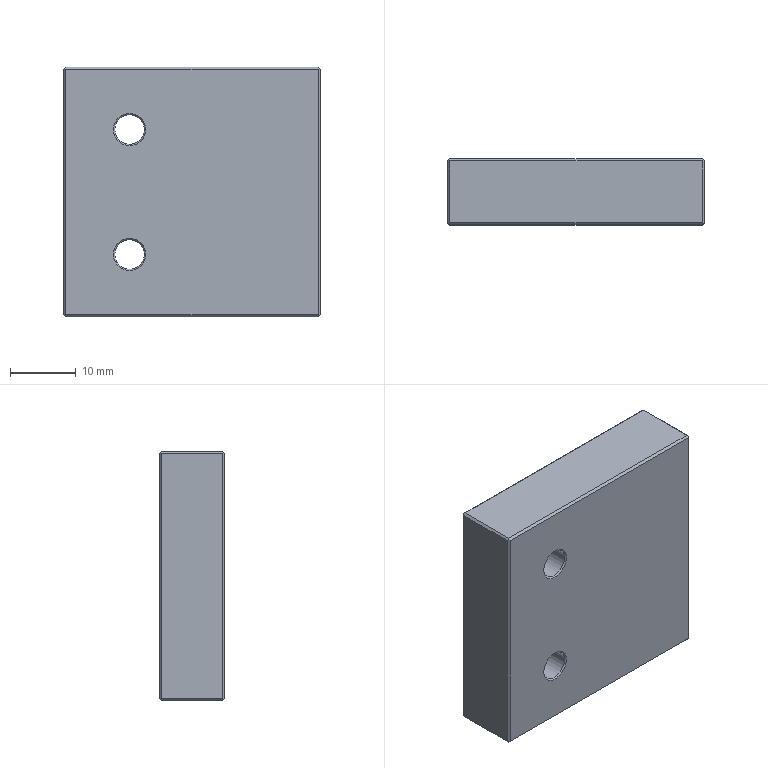Part | NX | 1 solid | 42 faces | box 39 x 10 x 38 mm | volume 14394 mm3 | plane 18 | cylinder 12 | cone 12 | commonest cylinder face diameters 2.5 x8 4.5 x4
STEP:
#1=CARTESIAN_POINT('',(-67.3,-35.,40.2));
#2=VERTEX_POINT('',#1);
#3=CARTESIAN_POINT('',(-67.3,-35.,2.8));
#4=VERTEX_POINT('',#3);
#5=CARTESIAN_POINT('',(-67.3,-35.,21.5));
#6=DIRECTION('',(0.,0.,-1.));
#7=VECTOR('',#6,1000.);
#8=LINE('',#5,#7);
#9=EDGE_CURVE('',#2,#4,#8,.T.);
#10=ORIENTED_EDGE('',*,*,#9,.F.);
#11=CARTESIAN_POINT('',(-105.7,-35.,40.2));
#12=VERTEX_POINT('',#11);
#13=CARTESIAN_POINT('',(-86.5,-35.,40.2));
#14=DIRECTION('',(-1.,0.,0.));
#15=VECTOR('',#14,1000.);
#16=LINE('',#13,#15);
#17=EDGE_CURVE('',#2,#12,#16,.T.);
#18=ORIENTED_EDGE('',*,*,#17,.T.);
#19=CARTESIAN_POINT('',(-105.7,-35.,2.8));
#20=VERTEX_POINT('',#19);
#21=CARTESIAN_POINT('',(-105.7,-35.,21.5));
#22=DIRECTION('',(0.,0.,-1.));
#23=VECTOR('',#22,1000.);
#24=LINE('',#21,#23);
#25=EDGE_CURVE('',#12,#20,#24,.T.);
#26=ORIENTED_EDGE('',*,*,#25,.T.);
#27=CARTESIAN_POINT('',(-86.5,-35.,2.8));
#28=DIRECTION('',(1.,0.,0.));
#29=VECTOR('',#28,1000.);
#30=LINE('',#27,#29);
#31=EDGE_CURVE('',#20,#4,#30,.T.);
#32=ORIENTED_EDGE('',*,*,#31,.T.);
#33=EDGE_LOOP('',(#10,#18,#26,#32));
#34=FACE_BOUND('',#33,.T.);
#35=CARTESIAN_POINT('',(-93.55,-35.,31.));
#36=VERTEX_POINT('',#35);
#37=CARTESIAN_POINT('',(-98.45,-35.,31.));
#38=VERTEX_POINT('',#37);
#39=CARTESIAN_POINT('',(-96.,-35.,31.));
#40=DIRECTION('',(0.,-1.,0.));
#41=DIRECTION('',(-1.,0.,0.));
#42=AXIS2_PLACEMENT_3D('',#39,#40,#41);
#43=CIRCLE('',#42,2.45);
#44=EDGE_CURVE('',#36,#38,#43,.T.);
#45=ORIENTED_EDGE('',*,*,#44,.F.);
#46=CARTESIAN_POINT('',(-96.,-35.,31.));
#47=DIRECTION('',(0.,-1.,0.));
#48=DIRECTION('',(-1.,0.,0.));
#49=AXIS2_PLACEMENT_3D('',#46,#47,#48);
#50=CIRCLE('',#49,2.45);
#51=EDGE_CURVE('',#38,#36,#50,.T.);
#52=ORIENTED_EDGE('',*,*,#51,.F.);
#53=EDGE_LOOP('',(#45,#52));
#54=FACE_BOUND('',#53,.T.);
#55=CARTESIAN_POINT('',(-93.55,-35.,12.));
#56=VERTEX_POINT('',#55);
#57=CARTESIAN_POINT('',(-98.45,-35.,12.));
#58=VERTEX_POINT('',#57);
#59=CARTESIAN_POINT('',(-96.,-35.,12.));
#60=DIRECTION('',(0.,-1.,0.));
#61=DIRECTION('',(-1.,0.,0.));
#62=AXIS2_PLACEMENT_3D('',#59,#60,#61);
#63=CIRCLE('',#62,2.45);
#64=EDGE_CURVE('',#56,#58,#63,.T.);
#65=ORIENTED_EDGE('',*,*,#64,.F.);
#66=CARTESIAN_POINT('',(-96.,-35.,12.));
#67=DIRECTION('',(0.,-1.,0.));
#68=DIRECTION('',(-1.,0.,0.));
#69=AXIS2_PLACEMENT_3D('',#66,#67,#68);
#70=CIRCLE('',#69,2.45);
#71=EDGE_CURVE('',#58,#56,#70,.T.);
#72=ORIENTED_EDGE('',*,*,#71,.F.);
#73=EDGE_LOOP('',(#65,#72));
#74=FACE_BOUND('',#73,.T.);
#75=CARTESIAN_POINT('',(0.,-35.,0.));
#76=DIRECTION('',(0.,1.,0.));
#77=DIRECTION('',(1.,0.,0.));
#78=AXIS2_PLACEMENT_3D('',#75,#76,#77);
#79=PLANE('',#78);
#80=ADVANCED_FACE('',(#34,#54,#74),#79,.F.);
#81=CARTESIAN_POINT('',(-105.7,-25.,2.8));
#82=VERTEX_POINT('',#81);
#83=CARTESIAN_POINT('',(-105.7,-25.,40.2));
#84=VERTEX_POINT('',#83);
#85=CARTESIAN_POINT('',(-105.7,-25.,21.5));
#86=DIRECTION('',(0.,0.,1.));
#87=VECTOR('',#86,1000.);
#88=LINE('',#85,#87);
#89=EDGE_CURVE('',#82,#84,#88,.T.);
#90=ORIENTED_EDGE('',*,*,#89,.T.);
#91=CARTESIAN_POINT('',(-67.3,-25.,40.2));
#92=VERTEX_POINT('',#91);
#93=CARTESIAN_POINT('',(-86.5,-25.,40.2));
#94=DIRECTION('',(-1.,0.,0.));
#95=VECTOR('',#94,1000.);
#96=LINE('',#93,#95);
#97=EDGE_CURVE('',#92,#84,#96,.T.);
#98=ORIENTED_EDGE('',*,*,#97,.F.);
#99=CARTESIAN_POINT('',(-67.3,-25.,2.8));
#100=VERTEX_POINT('',#99);
#101=CARTESIAN_POINT('',(-67.3,-25.,21.5));
#102=DIRECTION('',(0.,0.,1.));
#103=VECTOR('',#102,1000.);
#104=LINE('',#101,#103);
#105=EDGE_CURVE('',#100,#92,#104,.T.);
#106=ORIENTED_EDGE('',*,*,#105,.F.);
#107=CARTESIAN_POINT('',(-86.5,-25.,2.8));
#108=DIRECTION('',(1.,0.,0.));
#109=VECTOR('',#108,1000.);
#110=LINE('',#107,#109);
#111=EDGE_CURVE('',#82,#100,#110,.T.);
#112=ORIENTED_EDGE('',*,*,#111,.F.);
#113=EDGE_LOOP('',(#90,#98,#106,#112));
#114=FACE_BOUND('',#113,.T.);
#115=CARTESIAN_POINT('',(-93.75,-25.,12.));
#116=VERTEX_POINT('',#115);
#117=CARTESIAN_POINT('',(-98.25,-25.,12.));
#118=VERTEX_POINT('',#117);
#119=CARTESIAN_POINT('',(-96.,-25.,12.));
#120=DIRECTION('',(0.,-1.,0.));
#121=DIRECTION('',(-1.,0.,0.));
#122=AXIS2_PLACEMENT_3D('',#119,#120,#121);
#123=CIRCLE('',#122,2.25);
#124=EDGE_CURVE('',#116,#118,#123,.T.);
#125=ORIENTED_EDGE('',*,*,#124,.T.);
#126=CARTESIAN_POINT('',(-96.,-25.,12.));
#127=DIRECTION('',(0.,-1.,0.));
#128=DIRECTION('',(-1.,0.,0.));
#129=AXIS2_PLACEMENT_3D('',#126,#127,#128);
#130=CIRCLE('',#129,2.25);
#131=EDGE_CURVE('',#118,#116,#130,.T.);
#132=ORIENTED_EDGE('',*,*,#131,.T.);
#133=EDGE_LOOP('',(#125,#132));
#134=FACE_BOUND('',#133,.T.);
#135=CARTESIAN_POINT('',(-93.75,-25.,31.));
#136=VERTEX_POINT('',#135);
#137=CARTESIAN_POINT('',(-98.25,-25.,31.));
#138=VERTEX_POINT('',#137);
#139=CARTESIAN_POINT('',(-96.,-25.,31.));
#140=DIRECTION('',(0.,-1.,0.));
#141=DIRECTION('',(-1.,0.,0.));
#142=AXIS2_PLACEMENT_3D('',#139,#140,#141);
#143=CIRCLE('',#142,2.25);
#144=EDGE_CURVE('',#136,#138,#143,.T.);
#145=ORIENTED_EDGE('',*,*,#144,.T.);
#146=CARTESIAN_POINT('',(-96.,-25.,31.));
#147=DIRECTION('',(0.,-1.,0.));
#148=DIRECTION('',(-1.,0.,0.));
#149=AXIS2_PLACEMENT_3D('',#146,#147,#148);
#150=CIRCLE('',#149,2.25);
#151=EDGE_CURVE('',#138,#136,#150,.T.);
#152=ORIENTED_EDGE('',*,*,#151,.T.);
#153=EDGE_LOOP('',(#145,#152));
#154=FACE_BOUND('',#153,.T.);
#155=CARTESIAN_POINT('',(-8.5,-25.,1.2));
#156=DIRECTION('',(0.,-1.,0.));
#157=DIRECTION('',(-1.,0.,0.));
#158=AXIS2_PLACEMENT_3D('',#155,#156,#157);
#159=PLANE('',#158);
#160=ADVANCED_FACE('',(#114,#134,#154),#159,.F.);
#161=CARTESIAN_POINT('',(-106.,-25.3,2.8));
#162=VERTEX_POINT('',#161);
#163=CARTESIAN_POINT('',(-106.,-25.3,40.2));
#164=VERTEX_POINT('',#163);
#165=CARTESIAN_POINT('',(-106.,-25.3,21.5));
#166=DIRECTION('',(0.,0.,1.));
#167=VECTOR('',#166,1000.);
#168=LINE('',#165,#167);
#169=EDGE_CURVE('',#162,#164,#168,.T.);
#170=ORIENTED_EDGE('',*,*,#169,.F.);
#171=CARTESIAN_POINT('',(-106.,-34.7,2.8));
#172=VERTEX_POINT('',#171);
#173=CARTESIAN_POINT('',(-106.,-30.,2.8));
#174=DIRECTION('',(0.,1.,0.));
#175=VECTOR('',#174,1000.);
#176=LINE('',#173,#175);
#177=EDGE_CURVE('',#172,#162,#176,.T.);
#178=ORIENTED_EDGE('',*,*,#177,.F.);
#179=CARTESIAN_POINT('',(-106.,-34.7,40.2));
#180=VERTEX_POINT('',#179);
#181=CARTESIAN_POINT('',(-106.,-34.7,21.5));
#182=DIRECTION('',(0.,0.,-1.));
#183=VECTOR('',#182,1000.);
#184=LINE('',#181,#183);
#185=EDGE_CURVE('',#180,#172,#184,.T.);
#186=ORIENTED_EDGE('',*,*,#185,.F.);
#187=CARTESIAN_POINT('',(-106.,-30.,40.2));
#188=DIRECTION('',(0.,-1.,0.));
#189=VECTOR('',#188,1000.);
#190=LINE('',#187,#189);
#191=EDGE_CURVE('',#164,#180,#190,.T.);
#192=ORIENTED_EDGE('',*,*,#191,.F.);
#193=EDGE_LOOP('',(#170,#178,#186,#192));
#194=FACE_BOUND('',#193,.T.);
#195=CARTESIAN_POINT('',(-106.,0.,0.));
#196=DIRECTION('',(1.,0.,0.));
#197=DIRECTION('',(0.,1.,0.));
#198=AXIS2_PLACEMENT_3D('',#195,#196,#197);
#199=PLANE('',#198);
#200=ADVANCED_FACE('',(#194),#199,.F.);
#201=CARTESIAN_POINT('',(-67.3,-25.3,2.5));
#202=VERTEX_POINT('',#201);
#203=CARTESIAN_POINT('',(-67.3,-34.7,2.5));
#204=VERTEX_POINT('',#203);
#205=CARTESIAN_POINT('',(-67.3,0.,2.5));
#206=DIRECTION('',(0.,-1.,0.));
#207=VECTOR('',#206,1000.);
#208=LINE('',#205,#207);
#209=EDGE_CURVE('',#202,#204,#208,.T.);
#210=ORIENTED_EDGE('',*,*,#209,.T.);
#211=CARTESIAN_POINT('',(-105.7,-34.7,2.5));
#212=VERTEX_POINT('',#211);
#213=CARTESIAN_POINT('',(-86.5,-34.7,2.5));
#214=DIRECTION('',(1.,0.,0.));
#215=VECTOR('',#214,1000.);
#216=LINE('',#213,#215);
#217=EDGE_CURVE('',#212,#204,#216,.T.);
#218=ORIENTED_EDGE('',*,*,#217,.F.);
#219=CARTESIAN_POINT('',(-105.7,-25.3,2.5));
#220=VERTEX_POINT('',#219);
#221=CARTESIAN_POINT('',(-105.7,-30.,2.5));
#222=DIRECTION('',(0.,1.,0.));
#223=VECTOR('',#222,1000.);
#224=LINE('',#221,#223);
#225=EDGE_CURVE('',#212,#220,#224,.T.);
#226=ORIENTED_EDGE('',*,*,#225,.T.);
#227=CARTESIAN_POINT('',(-86.5,-25.3,2.5));
#228=DIRECTION('',(1.,0.,0.));
#229=VECTOR('',#228,1000.);
#230=LINE('',#227,#229);
#231=EDGE_CURVE('',#220,#202,#230,.T.);
#232=ORIENTED_EDGE('',*,*,#231,.T.);
#233=EDGE_LOOP('',(#210,#218,#226,#232));
#234=FACE_BOUND('',#233,.T.);
#235=CARTESIAN_POINT('',(-71.3,-31.,2.5));
#236=VERTEX_POINT('',#235);
#237=CARTESIAN_POINT('',(-74.7,-31.,2.5));
#238=VERTEX_POINT('',#237);
#239=CARTESIAN_POINT('',(-73.,-31.,2.5));
#240=DIRECTION('',(0.,0.,-1.));
#241=DIRECTION('',(-1.,0.,0.));
#242=AXIS2_PLACEMENT_3D('',#239,#240,#241);
#243=CIRCLE('',#242,1.7);
#244=EDGE_CURVE('',#236,#238,#243,.T.);
#245=ORIENTED_EDGE('',*,*,#244,.F.);
#246=CARTESIAN_POINT('',(-73.,-31.,2.5));
#247=DIRECTION('',(0.,0.,-1.));
#248=DIRECTION('',(-1.,0.,0.));
#249=AXIS2_PLACEMENT_3D('',#246,#247,#248);
#250=CIRCLE('',#249,1.7);
#251=EDGE_CURVE('',#238,#236,#250,.T.);
#252=ORIENTED_EDGE('',*,*,#251,.F.);
#253=EDGE_LOOP('',(#245,#252));
#254=FACE_BOUND('',#253,.T.);
#255=CARTESIAN_POINT('',(-78.3,-31.,2.5));
#256=VERTEX_POINT('',#255);
#257=CARTESIAN_POINT('',(-81.7,-31.,2.5));
#258=VERTEX_POINT('',#257);
#259=CARTESIAN_POINT('',(-80.,-31.,2.5));
#260=DIRECTION('',(0.,0.,-1.));
#261=DIRECTION('',(-1.,0.,0.));
#262=AXIS2_PLACEMENT_3D('',#259,#260,#261);
#263=CIRCLE('',#262,1.7);
#264=EDGE_CURVE('',#256,#258,#263,.T.);
#265=ORIENTED_EDGE('',*,*,#264,.F.);
#266=CARTESIAN_POINT('',(-80.,-31.,2.5));
#267=DIRECTION('',(0.,0.,-1.));
#268=DIRECTION('',(-1.,0.,0.));
#269=AXIS2_PLACEMENT_3D('',#266,#267,#268);
#270=CIRCLE('',#269,1.7);
#271=EDGE_CURVE('',#258,#256,#270,.T.);
#272=ORIENTED_EDGE('',*,*,#271,.F.);
#273=EDGE_LOOP('',(#265,#272));
#274=FACE_BOUND('',#273,.T.);
#275=CARTESIAN_POINT('',(-35.,0.,2.5));
#276=DIRECTION('',(0.,0.,1.));
#277=DIRECTION('',(1.,0.,0.));
#278=AXIS2_PLACEMENT_3D('',#275,#276,#277);
#279=PLANE('',#278);
#280=ADVANCED_FACE('',(#234,#254,#274),#279,.F.);
#281=CARTESIAN_POINT('',(-105.7,-25.3,40.5));
#282=VERTEX_POINT('',#281);
#283=CARTESIAN_POINT('',(-105.7,-34.7,40.5));
#284=VERTEX_POINT('',#283);
#285=CARTESIAN_POINT('',(-105.7,-30.,40.5));
#286=DIRECTION('',(0.,-1.,0.));
#287=VECTOR('',#286,1000.);
#288=LINE('',#285,#287);
#289=EDGE_CURVE('',#282,#284,#288,.T.);
#290=ORIENTED_EDGE('',*,*,#289,.F.);
#291=CARTESIAN_POINT('',(-105.85,-25.15,40.35));
#292=VERTEX_POINT('',#291);
#293=CARTESIAN_POINT('',(-131.,0.,15.2));
#294=DIRECTION('',(0.5774,-0.5774,0.5774));
#295=VECTOR('',#294,1000.);
#296=LINE('',#293,#295);
#297=EDGE_CURVE('',#292,#282,#296,.T.);
#298=ORIENTED_EDGE('',*,*,#297,.F.);
#299=CARTESIAN_POINT('',(-146.2,-65.5,0.));
#300=DIRECTION('',(0.5774,0.5774,0.5774));
#301=VECTOR('',#300,1000.);
#302=LINE('',#299,#301);
#303=EDGE_CURVE('',#164,#292,#302,.T.);
#304=ORIENTED_EDGE('',*,*,#303,.F.);
#305=ORIENTED_EDGE('',*,*,#191,.T.);
#306=CARTESIAN_POINT('',(-105.85,-34.85,40.35));
#307=VERTEX_POINT('',#306);
#308=CARTESIAN_POINT('',(-146.2,5.5,0.));
#309=DIRECTION('',(-0.5774,0.5774,-0.5774));
#310=VECTOR('',#309,1000.);
#311=LINE('',#308,#310);
#312=EDGE_CURVE('',#307,#180,#311,.T.);
#313=ORIENTED_EDGE('',*,*,#312,.F.);
#314=CARTESIAN_POINT('',(-146.2,-75.2,0.));
#315=DIRECTION('',(-0.5774,-0.5774,-0.5774));
#316=VECTOR('',#315,1000.);
#317=LINE('',#314,#316);
#318=EDGE_CURVE('',#284,#307,#317,.T.);
#319=ORIENTED_EDGE('',*,*,#318,.F.);
#320=EDGE_LOOP('',(#290,#298,#304,#305,#313,#319));
#321=FACE_BOUND('',#320,.T.);
#322=CARTESIAN_POINT('',(-105.85,-30.,40.35));
#323=DIRECTION('',(-0.7071,0.,0.7071));
#324=DIRECTION('',(0.,1.,0.));
#325=AXIS2_PLACEMENT_3D('',#322,#323,#324);
#326=PLANE('',#325);
#327=ADVANCED_FACE('',(#321),#326,.T.);
#328=ORIENTED_EDGE('',*,*,#289,.T.);
#329=CARTESIAN_POINT('',(-67.3,-34.7,40.5));
#330=VERTEX_POINT('',#329);
#331=CARTESIAN_POINT('',(-86.5,-34.7,40.5));
#332=DIRECTION('',(-1.,0.,0.));
#333=VECTOR('',#332,1000.);
#334=LINE('',#331,#333);
#335=EDGE_CURVE('',#330,#284,#334,.T.);
#336=ORIENTED_EDGE('',*,*,#335,.F.);
#337=CARTESIAN_POINT('',(-67.3,-25.3,40.5));
#338=VERTEX_POINT('',#337);
#339=CARTESIAN_POINT('',(-67.3,-30.,40.5));
#340=DIRECTION('',(0.,1.,0.));
#341=VECTOR('',#340,1000.);
#342=LINE('',#339,#341);
#343=EDGE_CURVE('',#330,#338,#342,.T.);
#344=ORIENTED_EDGE('',*,*,#343,.T.);
#345=CARTESIAN_POINT('',(-86.5,-25.3,40.5));
#346=DIRECTION('',(-1.,0.,0.));
#347=VECTOR('',#346,1000.);
#348=LINE('',#345,#347);
#349=EDGE_CURVE('',#338,#282,#348,.T.);
#350=ORIENTED_EDGE('',*,*,#349,.T.);
#351=EDGE_LOOP('',(#328,#336,#344,#350));
#352=FACE_BOUND('',#351,.T.);
#353=CARTESIAN_POINT('',(-20.5,7.5,40.5));
#354=DIRECTION('',(0.,0.,-1.));
#355=DIRECTION('',(0.,-1.,0.));
#356=AXIS2_PLACEMENT_3D('',#353,#354,#355);
#357=PLANE('',#356);
#358=ADVANCED_FACE('',(#352),#357,.F.);
#359=CARTESIAN_POINT('',(-78.75,-31.,2.76));
#360=VERTEX_POINT('',#359);
#361=CARTESIAN_POINT('',(-81.25,-31.,2.76));
#362=VERTEX_POINT('',#361);
#363=CARTESIAN_POINT('',(-80.,-31.,2.76));
#364=DIRECTION('',(0.,0.,-1.));
#365=DIRECTION('',(-1.,0.,0.));
#366=AXIS2_PLACEMENT_3D('',#363,#364,#365);
#367=CIRCLE('',#366,1.25);
#368=EDGE_CURVE('',#360,#362,#367,.T.);
#369=ORIENTED_EDGE('',*,*,#368,.T.);
#370=CARTESIAN_POINT('',(-81.25,-31.,8.5));
#371=VERTEX_POINT('',#370);
#372=CARTESIAN_POINT('',(-81.25,-31.,2.5));
#373=DIRECTION('',(0.,0.,-1.));
#374=VECTOR('',#373,1000.);
#375=LINE('',#372,#374);
#376=EDGE_CURVE('',#362,#371,#375,.F.);
#377=ORIENTED_EDGE('',*,*,#376,.T.);
#378=CARTESIAN_POINT('',(-78.75,-31.,8.5));
#379=VERTEX_POINT('',#378);
#380=CARTESIAN_POINT('',(-80.,-31.,8.5));
#381=DIRECTION('',(0.,0.,-1.));
#382=DIRECTION('',(-1.,0.,0.));
#383=AXIS2_PLACEMENT_3D('',#380,#381,#382);
#384=CIRCLE('',#383,1.25);
#385=EDGE_CURVE('',#379,#371,#384,.T.);
#386=ORIENTED_EDGE('',*,*,#385,.F.);
#387=CARTESIAN_POINT('',(-78.75,-31.,2.5));
#388=DIRECTION('',(0.,0.,-1.));
#389=VECTOR('',#388,1000.);
#390=LINE('',#387,#389);
#391=EDGE_CURVE('',#360,#379,#390,.F.);
#392=ORIENTED_EDGE('',*,*,#391,.F.);
#393=EDGE_LOOP('',(#369,#377,#386,#392));
#394=FACE_BOUND('',#393,.T.);
#395=CARTESIAN_POINT('',(-80.,-31.,2.5));
#396=DIRECTION('',(0.,0.,-1.));
#397=DIRECTION('',(-1.,0.,0.));
#398=AXIS2_PLACEMENT_3D('',#395,#396,#397);
#399=CYLINDRICAL_SURFACE('',#398,1.25);
#400=ADVANCED_FACE('',(#394),#399,.F.);
#401=ORIENTED_EDGE('',*,*,#385,.T.);
#402=CARTESIAN_POINT('',(-81.25,-31.,11.5));
#403=VERTEX_POINT('',#402);
#404=CARTESIAN_POINT('',(-81.25,-31.,2.5));
#405=DIRECTION('',(0.,0.,-1.));
#406=VECTOR('',#405,1000.);
#407=LINE('',#404,#406);
#408=EDGE_CURVE('',#371,#403,#407,.F.);
#409=ORIENTED_EDGE('',*,*,#408,.T.);
#410=CARTESIAN_POINT('',(-78.75,-31.,11.5));
#411=VERTEX_POINT('',#410);
#412=CARTESIAN_POINT('',(-80.,-31.,11.5));
#413=DIRECTION('',(0.,0.,-1.));
#414=DIRECTION('',(-1.,0.,0.));
#415=AXIS2_PLACEMENT_3D('',#412,#413,#414);
#416=CIRCLE('',#415,1.25);
#417=EDGE_CURVE('',#411,#403,#416,.T.);
#418=ORIENTED_EDGE('',*,*,#417,.F.);
#419=CARTESIAN_POINT('',(-78.75,-31.,2.5));
#420=DIRECTION('',(0.,0.,-1.));
#421=VECTOR('',#420,1000.);
#422=LINE('',#419,#421);
#423=EDGE_CURVE('',#379,#411,#422,.F.);
#424=ORIENTED_EDGE('',*,*,#423,.F.);
#425=EDGE_LOOP('',(#401,#409,#418,#424));
#426=FACE_BOUND('',#425,.T.);
#427=CARTESIAN_POINT('',(-80.,-31.,2.5));
#428=DIRECTION('',(0.,0.,-1.));
#429=DIRECTION('',(-1.,0.,0.));
#430=AXIS2_PLACEMENT_3D('',#427,#428,#429);
#431=CYLINDRICAL_SURFACE('',#430,1.25);
#432=ADVANCED_FACE('',(#426),#431,.F.);
#433=ORIENTED_EDGE('',*,*,#417,.T.);
#434=CARTESIAN_POINT('',(-80.,-31.,12.251));
#435=VERTEX_POINT('',#434);
#436=CARTESIAN_POINT('',(-81.25,-31.,11.5));
#437=DIRECTION('',(-0.8572,0.,-0.515));
#438=VECTOR('',#437,1000.);
#439=LINE('',#436,#438);
#440=EDGE_CURVE('',#435,#403,#439,.T.);
#441=ORIENTED_EDGE('',*,*,#440,.F.);
#442=CARTESIAN_POINT('',(-78.75,-31.,11.5));
#443=DIRECTION('',(0.8572,0.,-0.515));
#444=VECTOR('',#443,1000.);
#445=LINE('',#442,#444);
#446=EDGE_CURVE('',#435,#411,#445,.T.);
#447=ORIENTED_EDGE('',*,*,#446,.T.);
#448=EDGE_LOOP('',(#433,#441,#447));
#449=FACE_BOUND('',#448,.T.);
#450=CARTESIAN_POINT('',(-80.,-31.,11.5));
#451=DIRECTION('',(0.,0.,-1.));
#452=DIRECTION('',(-1.,0.,0.));
#453=AXIS2_PLACEMENT_3D('',#450,#451,#452);
#454=CONICAL_SURFACE('',#453,1.25,1.03);
#455=ADVANCED_FACE('',(#449),#454,.F.);
#456=CARTESIAN_POINT('',(-93.75,-34.8,31.));
#457=VERTEX_POINT('',#456);
#458=CARTESIAN_POINT('',(-98.25,-34.8,31.));
#459=VERTEX_POINT('',#458);
#460=CARTESIAN_POINT('',(-96.,-34.8,31.));
#461=DIRECTION('',(0.,-1.,0.));
#462=DIRECTION('',(-1.,0.,0.));
#463=AXIS2_PLACEMENT_3D('',#460,#461,#462);
#464=CIRCLE('',#463,2.25);
#465=EDGE_CURVE('',#457,#459,#464,.T.);
#466=ORIENTED_EDGE('',*,*,#465,.T.);
#467=CARTESIAN_POINT('',(-98.25,-35.,31.));
#468=DIRECTION('',(0.,-1.,0.));
#469=VECTOR('',#468,1000.);
#470=LINE('',#467,#469);
#471=EDGE_CURVE('',#459,#138,#470,.F.);
#472=ORIENTED_EDGE('',*,*,#471,.T.);
#473=ORIENTED_EDGE('',*,*,#144,.F.);
#474=CARTESIAN_POINT('',(-93.75,-35.,31.));
#475=DIRECTION('',(0.,-1.,0.));
#476=VECTOR('',#475,1000.);
#477=LINE('',#474,#476);
#478=EDGE_CURVE('',#457,#136,#477,.F.);
#479=ORIENTED_EDGE('',*,*,#478,.F.);
#480=EDGE_LOOP('',(#466,#472,#473,#479));
#481=FACE_BOUND('',#480,.T.);
#482=CARTESIAN_POINT('',(-96.,-35.,31.));
#483=DIRECTION('',(0.,-1.,0.));
#484=DIRECTION('',(-1.,0.,0.));
#485=AXIS2_PLACEMENT_3D('',#482,#483,#484);
#486=CYLINDRICAL_SURFACE('',#485,2.25);
#487=ADVANCED_FACE('',(#481),#486,.F.);
#488=CARTESIAN_POINT('',(-71.75,-31.,2.76));
#489=VERTEX_POINT('',#488);
#490=CARTESIAN_POINT('',(-74.25,-31.,2.76));
#491=VERTEX_POINT('',#490);
#492=CARTESIAN_POINT('',(-73.,-31.,2.76));
#493=DIRECTION('',(0.,0.,-1.));
#494=DIRECTION('',(-1.,0.,0.));
#495=AXIS2_PLACEMENT_3D('',#492,#493,#494);
#496=CIRCLE('',#495,1.25);
#497=EDGE_CURVE('',#489,#491,#496,.T.);
#498=ORIENTED_EDGE('',*,*,#497,.T.);
#499=CARTESIAN_POINT('',(-74.25,-31.,8.5));
#500=VERTEX_POINT('',#499);
#501=CARTESIAN_POINT('',(-74.25,-31.,2.5));
#502=DIRECTION('',(0.,0.,-1.));
#503=VECTOR('',#502,1000.);
#504=LINE('',#501,#503);
#505=EDGE_CURVE('',#491,#500,#504,.F.);
#506=ORIENTED_EDGE('',*,*,#505,.T.);
#507=CARTESIAN_POINT('',(-71.75,-31.,8.5));
#508=VERTEX_POINT('',#507);
#509=CARTESIAN_POINT('',(-73.,-31.,8.5));
#510=DIRECTION('',(0.,0.,-1.));
#511=DIRECTION('',(-1.,0.,0.));
#512=AXIS2_PLACEMENT_3D('',#509,#510,#511);
#513=CIRCLE('',#512,1.25);
#514=EDGE_CURVE('',#508,#500,#513,.T.);
#515=ORIENTED_EDGE('',*,*,#514,.F.);
#516=CARTESIAN_POINT('',(-71.75,-31.,2.5));
#517=DIRECTION('',(0.,0.,-1.));
#518=VECTOR('',#517,1000.);
#519=LINE('',#516,#518);
#520=EDGE_CURVE('',#489,#508,#519,.F.);
#521=ORIENTED_EDGE('',*,*,#520,.F.);
#522=EDGE_LOOP('',(#498,#506,#515,#521));
#523=FACE_BOUND('',#522,.T.);
#524=CARTESIAN_POINT('',(-73.,-31.,2.5));
#525=DIRECTION('',(0.,0.,-1.));
#526=DIRECTION('',(-1.,0.,0.));
#527=AXIS2_PLACEMENT_3D('',#524,#525,#526);
#528=CYLINDRICAL_SURFACE('',#527,1.25);
#529=ADVANCED_FACE('',(#523),#528,.F.);
#530=ORIENTED_EDGE('',*,*,#514,.T.);
#531=CARTESIAN_POINT('',(-74.25,-31.,11.5));
#532=VERTEX_POINT('',#531);
#533=CARTESIAN_POINT('',(-74.25,-31.,2.5));
#534=DIRECTION('',(0.,0.,-1.));
#535=VECTOR('',#534,1000.);
#536=LINE('',#533,#535);
#537=EDGE_CURVE('',#500,#532,#536,.F.);
#538=ORIENTED_EDGE('',*,*,#537,.T.);
#539=CARTESIAN_POINT('',(-71.75,-31.,11.5));
#540=VERTEX_POINT('',#539);
#541=CARTESIAN_POINT('',(-73.,-31.,11.5));
#542=DIRECTION('',(0.,0.,-1.));
#543=DIRECTION('',(-1.,0.,0.));
#544=AXIS2_PLACEMENT_3D('',#541,#542,#543);
#545=CIRCLE('',#544,1.25);
#546=EDGE_CURVE('',#540,#532,#545,.T.);
#547=ORIENTED_EDGE('',*,*,#546,.F.);
#548=CARTESIAN_POINT('',(-71.75,-31.,2.5));
#549=DIRECTION('',(0.,0.,-1.));
#550=VECTOR('',#549,1000.);
#551=LINE('',#548,#550);
#552=EDGE_CURVE('',#508,#540,#551,.F.);
#553=ORIENTED_EDGE('',*,*,#552,.F.);
#554=EDGE_LOOP('',(#530,#538,#547,#553));
#555=FACE_BOUND('',#554,.T.);
#556=CARTESIAN_POINT('',(-73.,-31.,2.5));
#557=DIRECTION('',(0.,0.,-1.));
#558=DIRECTION('',(-1.,0.,0.));
#559=AXIS2_PLACEMENT_3D('',#556,#557,#558);
#560=CYLINDRICAL_SURFACE('',#559,1.25);
#561=ADVANCED_FACE('',(#555),#560,.F.);
#562=ORIENTED_EDGE('',*,*,#546,.T.);
#563=CARTESIAN_POINT('',(-73.,-31.,12.251));
#564=VERTEX_POINT('',#563);
#565=CARTESIAN_POINT('',(-74.25,-31.,11.5));
#566=DIRECTION('',(-0.8572,0.,-0.515));
#567=VECTOR('',#566,1000.);
#568=LINE('',#565,#567);
#569=EDGE_CURVE('',#564,#532,#568,.T.);
#570=ORIENTED_EDGE('',*,*,#569,.F.);
#571=CARTESIAN_POINT('',(-71.75,-31.,11.5));
#572=DIRECTION('',(0.8572,0.,-0.515));
#573=VECTOR('',#572,1000.);
#574=LINE('',#571,#573);
#575=EDGE_CURVE('',#564,#540,#574,.T.);
#576=ORIENTED_EDGE('',*,*,#575,.T.);
#577=EDGE_LOOP('',(#562,#570,#576));
#578=FACE_BOUND('',#577,.T.);
#579=CARTESIAN_POINT('',(-73.,-31.,11.5));
#580=DIRECTION('',(0.,0.,-1.));
#581=DIRECTION('',(-1.,0.,0.));
#582=AXIS2_PLACEMENT_3D('',#579,#580,#581);
#583=CONICAL_SURFACE('',#582,1.25,1.03);
#584=ADVANCED_FACE('',(#578),#583,.F.);
#585=CARTESIAN_POINT('',(-67.,-25.3,2.8));
#586=VERTEX_POINT('',#585);
#587=CARTESIAN_POINT('',(-67.,-34.7,2.8));
#588=VERTEX_POINT('',#587);
#589=CARTESIAN_POINT('',(-67.,0.,2.8));
#590=DIRECTION('',(0.,-1.,0.));
#591=VECTOR('',#590,1000.);
#592=LINE('',#589,#591);
#593=EDGE_CURVE('',#586,#588,#592,.T.);
#594=ORIENTED_EDGE('',*,*,#593,.F.);
#595=CARTESIAN_POINT('',(-67.,-25.3,40.2));
#596=VERTEX_POINT('',#595);
#597=CARTESIAN_POINT('',(-67.,-25.3,0.));
#598=DIRECTION('',(0.,0.,-1.));
#599=VECTOR('',#598,1000.);
#600=LINE('',#597,#599);
#601=EDGE_CURVE('',#596,#586,#600,.T.);
#602=ORIENTED_EDGE('',*,*,#601,.F.);
#603=CARTESIAN_POINT('',(-67.,-34.7,40.2));
#604=VERTEX_POINT('',#603);
#605=CARTESIAN_POINT('',(-67.,-30.,40.2));
#606=DIRECTION('',(0.,1.,0.));
#607=VECTOR('',#606,1000.);
#608=LINE('',#605,#607);
#609=EDGE_CURVE('',#604,#596,#608,.T.);
#610=ORIENTED_EDGE('',*,*,#609,.F.);
#611=CARTESIAN_POINT('',(-67.,-34.7,21.5));
#612=DIRECTION('',(0.,0.,-1.));
#613=VECTOR('',#612,1000.);
#614=LINE('',#611,#613);
#615=EDGE_CURVE('',#604,#588,#614,.T.);
#616=ORIENTED_EDGE('',*,*,#615,.T.);
#617=EDGE_LOOP('',(#594,#602,#610,#616));
#618=FACE_BOUND('',#617,.T.);
#619=CARTESIAN_POINT('',(-67.,-38.5,5.));
#620=DIRECTION('',(1.,0.,0.));
#621=DIRECTION('',(0.,1.,0.));
#622=AXIS2_PLACEMENT_3D('',#619,#620,#621);
#623=PLANE('',#622);
#624=ADVANCED_FACE('',(#618),#623,.T.);
#625=ORIENTED_EDGE('',*,*,#9,.T.);
#626=CARTESIAN_POINT('',(-67.15,-34.85,2.65));
#627=VERTEX_POINT('',#626);
#628=CARTESIAN_POINT('',(0.,32.3,-64.5));
#629=DIRECTION('',(0.5774,0.5774,-0.5774));
#630=VECTOR('',#629,1000.);
#631=LINE('',#628,#630);
#632=EDGE_CURVE('',#4,#627,#631,.T.);
#633=ORIENTED_EDGE('',*,*,#632,.T.);
#634=CARTESIAN_POINT('',(-69.8,-37.5,0.));
#635=DIRECTION('',(-0.5774,-0.5774,-0.5774));
#636=VECTOR('',#635,1000.);
#637=LINE('',#634,#636);
#638=EDGE_CURVE('',#588,#627,#637,.T.);
#639=ORIENTED_EDGE('',*,*,#638,.F.);
#640=ORIENTED_EDGE('',*,*,#615,.F.);
#641=CARTESIAN_POINT('',(-67.15,-34.85,40.35));
#642=VERTEX_POINT('',#641);
#643=CARTESIAN_POINT('',(-26.8,5.5,0.));
#644=DIRECTION('',(0.5774,0.5774,-0.5774));
#645=VECTOR('',#644,1000.);
#646=LINE('',#643,#645);
#647=EDGE_CURVE('',#642,#604,#646,.T.);
#648=ORIENTED_EDGE('',*,*,#647,.F.);
#649=CARTESIAN_POINT('',(0.,32.3,107.5));
#650=DIRECTION('',(-0.5774,-0.5774,-0.5774));
#651=VECTOR('',#650,1000.);
#652=LINE('',#649,#651);
#653=EDGE_CURVE('',#642,#2,#652,.T.);
#654=ORIENTED_EDGE('',*,*,#653,.T.);
#655=EDGE_LOOP('',(#625,#633,#639,#640,#648,#654));
#656=FACE_BOUND('',#655,.T.);
#657=CARTESIAN_POINT('',(-67.15,-34.85,21.5));
#658=DIRECTION('',(-0.7071,0.7071,0.));
#659=DIRECTION('',(0.,0.,1.));
#660=AXIS2_PLACEMENT_3D('',#657,#658,#659);
#661=PLANE('',#660);
#662=ADVANCED_FACE('',(#656),#661,.F.);
#663=ORIENTED_EDGE('',*,*,#593,.T.);
#664=ORIENTED_EDGE('',*,*,#638,.T.);
#665=CARTESIAN_POINT('',(-69.8,-32.2,0.));
#666=DIRECTION('',(0.5774,-0.5774,0.5774));
#667=VECTOR('',#666,1000.);
#668=LINE('',#665,#667);
#669=EDGE_CURVE('',#204,#627,#668,.T.);
#670=ORIENTED_EDGE('',*,*,#669,.F.);
#671=ORIENTED_EDGE('',*,*,#209,.F.);
#672=CARTESIAN_POINT('',(-67.15,-25.15,2.65));
#673=VERTEX_POINT('',#672);
#674=CARTESIAN_POINT('',(-69.8,-27.8,0.));
#675=DIRECTION('',(-0.5774,-0.5774,-0.5774));
#676=VECTOR('',#675,1000.);
#677=LINE('',#674,#676);
#678=EDGE_CURVE('',#673,#202,#677,.T.);
#679=ORIENTED_EDGE('',*,*,#678,.F.);
#680=CARTESIAN_POINT('',(-92.3,0.,-22.5));
#681=DIRECTION('',(0.5774,-0.5774,0.5774));
#682=VECTOR('',#681,1000.);
#683=LINE('',#680,#682);
#684=EDGE_CURVE('',#673,#586,#683,.T.);
#685=ORIENTED_EDGE('',*,*,#684,.T.);
#686=EDGE_LOOP('',(#663,#664,#670,#671,#679,#685));
#687=FACE_BOUND('',#686,.T.);
#688=CARTESIAN_POINT('',(-67.15,-27.625,2.65));
#689=DIRECTION('',(0.7071,0.,-0.7071));
#690=DIRECTION('',(0.,-1.,0.));
#691=AXIS2_PLACEMENT_3D('',#688,#689,#690);
#692=PLANE('',#691);
#693=ADVANCED_FACE('',(#687),#692,.T.);
#694=CARTESIAN_POINT('',(-93.75,-34.8,12.));
#695=VERTEX_POINT('',#694);
#696=CARTESIAN_POINT('',(-98.25,-34.8,12.));
#697=VERTEX_POINT('',#696);
#698=CARTESIAN_POINT('',(-96.,-34.8,12.));
#699=DIRECTION('',(0.,-1.,0.));
#700=DIRECTION('',(-1.,0.,0.));
#701=AXIS2_PLACEMENT_3D('',#698,#699,#700);
#702=CIRCLE('',#701,2.25);
#703=EDGE_CURVE('',#695,#697,#702,.T.);
#704=ORIENTED_EDGE('',*,*,#703,.T.);
#705=CARTESIAN_POINT('',(-98.25,-35.,12.));
#706=DIRECTION('',(0.,-1.,0.));
#707=VECTOR('',#706,1000.);
#708=LINE('',#705,#707);
#709=EDGE_CURVE('',#697,#118,#708,.F.);
#710=ORIENTED_EDGE('',*,*,#709,.T.);
#711=ORIENTED_EDGE('',*,*,#124,.F.);
#712=CARTESIAN_POINT('',(-93.75,-35.,12.));
#713=DIRECTION('',(0.,-1.,0.));
#714=VECTOR('',#713,1000.);
#715=LINE('',#712,#714);
#716=EDGE_CURVE('',#695,#116,#715,.F.);
#717=ORIENTED_EDGE('',*,*,#716,.F.);
#718=EDGE_LOOP('',(#704,#710,#711,#717));
#719=FACE_BOUND('',#718,.T.);
#720=CARTESIAN_POINT('',(-96.,-35.,12.));
#721=DIRECTION('',(0.,-1.,0.));
#722=DIRECTION('',(-1.,0.,0.));
#723=AXIS2_PLACEMENT_3D('',#720,#721,#722);
#724=CYLINDRICAL_SURFACE('',#723,2.25);
#725=ADVANCED_FACE('',(#719),#724,.F.);
#726=ORIENTED_EDGE('',*,*,#368,.F.);
#727=CARTESIAN_POINT('',(-78.75,-31.,2.76));
#728=DIRECTION('',(0.866,0.,-0.5));
#729=VECTOR('',#728,1000.);
#730=LINE('',#727,#729);
#731=EDGE_CURVE('',#256,#360,#730,.F.);
#732=ORIENTED_EDGE('',*,*,#731,.F.);
#733=ORIENTED_EDGE('',*,*,#264,.T.);
#734=CARTESIAN_POINT('',(-81.25,-31.,2.76));
#735=DIRECTION('',(-0.866,0.,-0.5));
#736=VECTOR('',#735,1000.);
#737=LINE('',#734,#736);
#738=EDGE_CURVE('',#258,#362,#737,.F.);
#739=ORIENTED_EDGE('',*,*,#738,.T.);
#740=EDGE_LOOP('',(#726,#732,#733,#739));
#741=FACE_BOUND('',#740,.T.);
#742=CARTESIAN_POINT('',(-80.,-31.,2.76));
#743=DIRECTION('',(0.,0.,-1.));
#744=DIRECTION('',(-1.,0.,0.));
#745=AXIS2_PLACEMENT_3D('',#742,#743,#744);
#746=CONICAL_SURFACE('',#745,1.25,1.047);
#747=ADVANCED_FACE('',(#741),#746,.F.);
#748=ORIENTED_EDGE('',*,*,#703,.F.);
#749=CARTESIAN_POINT('',(-93.75,-34.8,12.));
#750=DIRECTION('',(0.7071,-0.7071,0.));
#751=VECTOR('',#750,1000.);
#752=LINE('',#749,#751);
#753=EDGE_CURVE('',#56,#695,#752,.F.);
#754=ORIENTED_EDGE('',*,*,#753,.F.);
#755=ORIENTED_EDGE('',*,*,#64,.T.);
#756=CARTESIAN_POINT('',(-98.25,-34.8,12.));
#757=DIRECTION('',(-0.7071,-0.7071,0.));
#758=VECTOR('',#757,1000.);
#759=LINE('',#756,#758);
#760=EDGE_CURVE('',#58,#697,#759,.F.);
#761=ORIENTED_EDGE('',*,*,#760,.T.);
#762=EDGE_LOOP('',(#748,#754,#755,#761));
#763=FACE_BOUND('',#762,.T.);
#764=CARTESIAN_POINT('',(-96.,-34.8,12.));
#765=DIRECTION('',(0.,-1.,0.));
#766=DIRECTION('',(-1.,0.,0.));
#767=AXIS2_PLACEMENT_3D('',#764,#765,#766);
#768=CONICAL_SURFACE('',#767,2.25,0.7854);
#769=ADVANCED_FACE('',(#763),#768,.F.);
#770=ORIENTED_EDGE('',*,*,#497,.F.);
#771=CARTESIAN_POINT('',(-71.75,-31.,2.76));
#772=DIRECTION('',(0.866,0.,-0.5));
#773=VECTOR('',#772,1000.);
#774=LINE('',#771,#773);
#775=EDGE_CURVE('',#236,#489,#774,.F.);
#776=ORIENTED_EDGE('',*,*,#775,.F.);
#777=ORIENTED_EDGE('',*,*,#244,.T.);
#778=CARTESIAN_POINT('',(-74.25,-31.,2.76));
#779=DIRECTION('',(-0.866,0.,-0.5));
#780=VECTOR('',#779,1000.);
#781=LINE('',#778,#780);
#782=EDGE_CURVE('',#238,#491,#781,.F.);
#783=ORIENTED_EDGE('',*,*,#782,.T.);
#784=EDGE_LOOP('',(#770,#776,#777,#783));
#785=FACE_BOUND('',#784,.T.);
#786=CARTESIAN_POINT('',(-73.,-31.,2.76));
#787=DIRECTION('',(0.,0.,-1.));
#788=DIRECTION('',(-1.,0.,0.));
#789=AXIS2_PLACEMENT_3D('',#786,#787,#788);
#790=CONICAL_SURFACE('',#789,1.25,1.047);
#791=ADVANCED_FACE('',(#785),#790,.F.);
#792=ORIENTED_EDGE('',*,*,#465,.F.);
#793=CARTESIAN_POINT('',(-93.75,-34.8,31.));
#794=DIRECTION('',(0.7071,-0.7071,0.));
#795=VECTOR('',#794,1000.);
#796=LINE('',#793,#795);
#797=EDGE_CURVE('',#36,#457,#796,.F.);
#798=ORIENTED_EDGE('',*,*,#797,.F.);
#799=ORIENTED_EDGE('',*,*,#44,.T.);
#800=CARTESIAN_POINT('',(-98.25,-34.8,31.));
#801=DIRECTION('',(-0.7071,-0.7071,0.));
#802=VECTOR('',#801,1000.);
#803=LINE('',#800,#802);
#804=EDGE_CURVE('',#38,#459,#803,.F.);
#805=ORIENTED_EDGE('',*,*,#804,.T.);
#806=EDGE_LOOP('',(#792,#798,#799,#805));
#807=FACE_BOUND('',#806,.T.);
#808=CARTESIAN_POINT('',(-96.,-34.8,31.));
#809=DIRECTION('',(0.,-1.,0.));
#810=DIRECTION('',(-1.,0.,0.));
#811=AXIS2_PLACEMENT_3D('',#808,#809,#810);
#812=CONICAL_SURFACE('',#811,2.25,0.7854);
#813=ADVANCED_FACE('',(#807),#812,.F.);
#814=ORIENTED_EDGE('',*,*,#609,.T.);
#815=CARTESIAN_POINT('',(-67.15,-25.15,40.35));
#816=VERTEX_POINT('',#815);
#817=CARTESIAN_POINT('',(-92.3,0.,65.5));
#818=DIRECTION('',(-0.5774,0.5774,0.5774));
#819=VECTOR('',#818,1000.);
#820=LINE('',#817,#819);
#821=EDGE_CURVE('',#596,#816,#820,.T.);
#822=ORIENTED_EDGE('',*,*,#821,.T.);
#823=CARTESIAN_POINT('',(0.,42.,-26.8));
#824=DIRECTION('',(0.5774,0.5774,-0.5774));
#825=VECTOR('',#824,1000.);
#826=LINE('',#823,#825);
#827=EDGE_CURVE('',#338,#816,#826,.T.);
#828=ORIENTED_EDGE('',*,*,#827,.F.);
#829=ORIENTED_EDGE('',*,*,#343,.F.);
#830=CARTESIAN_POINT('',(-26.8,-75.2,0.));
#831=DIRECTION('',(-0.5774,0.5774,0.5774));
#832=VECTOR('',#831,1000.);
#833=LINE('',#830,#832);
#834=EDGE_CURVE('',#642,#330,#833,.T.);
#835=ORIENTED_EDGE('',*,*,#834,.F.);
#836=ORIENTED_EDGE('',*,*,#647,.T.);
#837=EDGE_LOOP('',(#814,#822,#828,#829,#835,#836));
#838=FACE_BOUND('',#837,.T.);
#839=CARTESIAN_POINT('',(-67.15,-30.,40.35));
#840=DIRECTION('',(-0.7071,0.,-0.7071));
#841=DIRECTION('',(-0.7071,0.,0.7071));
#842=AXIS2_PLACEMENT_3D('',#839,#840,#841);
#843=PLANE('',#842);
#844=ADVANCED_FACE('',(#838),#843,.F.);
#845=ORIENTED_EDGE('',*,*,#105,.T.);
#846=CARTESIAN_POINT('',(-92.3,0.,15.2));
#847=DIRECTION('',(-0.5774,0.5774,-0.5774));
#848=VECTOR('',#847,1000.);
#849=LINE('',#846,#848);
#850=EDGE_CURVE('',#816,#92,#849,.T.);
#851=ORIENTED_EDGE('',*,*,#850,.F.);
#852=ORIENTED_EDGE('',*,*,#821,.F.);
#853=ORIENTED_EDGE('',*,*,#601,.T.);
#854=ORIENTED_EDGE('',*,*,#684,.F.);
#855=CARTESIAN_POINT('',(-92.3,0.,27.8));
#856=DIRECTION('',(0.5774,-0.5774,-0.5774));
#857=VECTOR('',#856,1000.);
#858=LINE('',#855,#857);
#859=EDGE_CURVE('',#100,#673,#858,.T.);
#860=ORIENTED_EDGE('',*,*,#859,.F.);
#861=EDGE_LOOP('',(#845,#851,#852,#853,#854,#860));
#862=FACE_BOUND('',#861,.T.);
#863=CARTESIAN_POINT('',(-67.15,-25.15,21.5));
#864=DIRECTION('',(-0.7071,-0.7071,0.));
#865=DIRECTION('',(-0.7071,0.7071,0.));
#866=AXIS2_PLACEMENT_3D('',#863,#864,#865);
#867=PLANE('',#866);
#868=ADVANCED_FACE('',(#862),#867,.F.);
#869=ORIENTED_EDGE('',*,*,#349,.F.);
#870=ORIENTED_EDGE('',*,*,#827,.T.);
#871=ORIENTED_EDGE('',*,*,#850,.T.);
#872=ORIENTED_EDGE('',*,*,#97,.T.);
#873=CARTESIAN_POINT('',(-65.5,15.2,0.));
#874=DIRECTION('',(-0.5774,-0.5774,0.5774));
#875=VECTOR('',#874,1000.);
#876=LINE('',#873,#875);
#877=EDGE_CURVE('',#84,#292,#876,.T.);
#878=ORIENTED_EDGE('',*,*,#877,.T.);
#879=ORIENTED_EDGE('',*,*,#297,.T.);
#880=EDGE_LOOP('',(#869,#870,#871,#872,#878,#879));
#881=FACE_BOUND('',#880,.T.);
#882=CARTESIAN_POINT('',(-86.5,-25.15,40.35));
#883=DIRECTION('',(0.,0.7071,0.7071));
#884=DIRECTION('',(1.,0.,0.));
#885=AXIS2_PLACEMENT_3D('',#882,#883,#884);
#886=PLANE('',#885);
#887=ADVANCED_FACE('',(#881),#886,.T.);
#888=ORIENTED_EDGE('',*,*,#89,.F.);
#889=CARTESIAN_POINT('',(-105.85,-25.15,2.65));
#890=VERTEX_POINT('',#889);
#891=CARTESIAN_POINT('',(-108.5,-27.8,0.));
#892=DIRECTION('',(-0.5774,-0.5774,-0.5774));
#893=VECTOR('',#892,1000.);
#894=LINE('',#891,#893);
#895=EDGE_CURVE('',#82,#890,#894,.T.);
#896=ORIENTED_EDGE('',*,*,#895,.T.);
#897=CARTESIAN_POINT('',(-103.2,-22.5,0.));
#898=DIRECTION('',(-0.5774,-0.5774,0.5774));
#899=VECTOR('',#898,1000.);
#900=LINE('',#897,#899);
#901=EDGE_CURVE('',#890,#162,#900,.T.);
#902=ORIENTED_EDGE('',*,*,#901,.T.);
#903=ORIENTED_EDGE('',*,*,#169,.T.);
#904=ORIENTED_EDGE('',*,*,#303,.T.);
#905=ORIENTED_EDGE('',*,*,#877,.F.);
#906=EDGE_LOOP('',(#888,#896,#902,#903,#904,#905));
#907=FACE_BOUND('',#906,.T.);
#908=CARTESIAN_POINT('',(-105.85,-25.15,21.5));
#909=DIRECTION('',(-0.7071,0.7071,0.));
#910=DIRECTION('',(0.,0.,1.));
#911=AXIS2_PLACEMENT_3D('',#908,#909,#910);
#912=PLANE('',#911);
#913=ADVANCED_FACE('',(#907),#912,.T.);
#914=ORIENTED_EDGE('',*,*,#231,.F.);
#915=CARTESIAN_POINT('',(-131.,0.,27.8));
#916=DIRECTION('',(-0.5774,0.5774,0.5774));
#917=VECTOR('',#916,1000.);
#918=LINE('',#915,#917);
#919=EDGE_CURVE('',#220,#890,#918,.T.);
#920=ORIENTED_EDGE('',*,*,#919,.T.);
#921=ORIENTED_EDGE('',*,*,#895,.F.);
#922=ORIENTED_EDGE('',*,*,#111,.T.);
#923=ORIENTED_EDGE('',*,*,#859,.T.);
#924=ORIENTED_EDGE('',*,*,#678,.T.);
#925=EDGE_LOOP('',(#914,#920,#921,#922,#923,#924));
#926=FACE_BOUND('',#925,.T.);
#927=CARTESIAN_POINT('',(-86.5,-25.15,2.65));
#928=DIRECTION('',(0.,0.7071,-0.7071));
#929=DIRECTION('',(-1.,0.,0.));
#930=AXIS2_PLACEMENT_3D('',#927,#928,#929);
#931=PLANE('',#930);
#932=ADVANCED_FACE('',(#926),#931,.T.);
#933=ORIENTED_EDGE('',*,*,#225,.F.);
#934=CARTESIAN_POINT('',(-105.85,-34.85,2.65));
#935=VERTEX_POINT('',#934);
#936=CARTESIAN_POINT('',(-103.2,-32.2,0.));
#937=DIRECTION('',(-0.5774,-0.5774,0.5774));
#938=VECTOR('',#937,1000.);
#939=LINE('',#936,#938);
#940=EDGE_CURVE('',#212,#935,#939,.T.);
#941=ORIENTED_EDGE('',*,*,#940,.T.);
#942=CARTESIAN_POINT('',(-103.2,-37.5,0.));
#943=DIRECTION('',(-0.5774,0.5774,0.5774));
#944=VECTOR('',#943,1000.);
#945=LINE('',#942,#944);
#946=EDGE_CURVE('',#935,#172,#945,.T.);
#947=ORIENTED_EDGE('',*,*,#946,.T.);
#948=ORIENTED_EDGE('',*,*,#177,.T.);
#949=ORIENTED_EDGE('',*,*,#901,.F.);
#950=ORIENTED_EDGE('',*,*,#919,.F.);
#951=EDGE_LOOP('',(#933,#941,#947,#948,#949,#950));
#952=FACE_BOUND('',#951,.T.);
#953=CARTESIAN_POINT('',(-105.85,-30.,2.65));
#954=DIRECTION('',(-0.7071,0.,-0.7071));
#955=DIRECTION('',(-0.7071,0.,0.7071));
#956=AXIS2_PLACEMENT_3D('',#953,#954,#955);
#957=PLANE('',#956);
#958=ADVANCED_FACE('',(#952),#957,.T.);
#959=ORIENTED_EDGE('',*,*,#31,.F.);
#960=CARTESIAN_POINT('',(-108.5,-32.2,0.));
#961=DIRECTION('',(-0.5774,0.5774,-0.5774));
#962=VECTOR('',#961,1000.);
#963=LINE('',#960,#962);
#964=EDGE_CURVE('',#20,#935,#963,.T.);
#965=ORIENTED_EDGE('',*,*,#964,.T.);
#966=ORIENTED_EDGE('',*,*,#940,.F.);
#967=ORIENTED_EDGE('',*,*,#217,.T.);
#968=ORIENTED_EDGE('',*,*,#669,.T.);
#969=ORIENTED_EDGE('',*,*,#632,.F.);
#970=EDGE_LOOP('',(#959,#965,#966,#967,#968,#969));
#971=FACE_BOUND('',#970,.T.);
#972=CARTESIAN_POINT('',(-86.5,-34.85,2.65));
#973=DIRECTION('',(0.,-0.7071,-0.7071));
#974=DIRECTION('',(0.,0.7071,-0.7071));
#975=AXIS2_PLACEMENT_3D('',#972,#973,#974);
#976=PLANE('',#975);
#977=ADVANCED_FACE('',(#971),#976,.T.);
#978=ORIENTED_EDGE('',*,*,#25,.F.);
#979=CARTESIAN_POINT('',(-65.5,-75.2,0.));
#980=DIRECTION('',(-0.5774,0.5774,0.5774));
#981=VECTOR('',#980,1000.);
#982=LINE('',#979,#981);
#983=EDGE_CURVE('',#12,#307,#982,.T.);
#984=ORIENTED_EDGE('',*,*,#983,.T.);
#985=ORIENTED_EDGE('',*,*,#312,.T.);
#986=ORIENTED_EDGE('',*,*,#185,.T.);
#987=ORIENTED_EDGE('',*,*,#946,.F.);
#988=ORIENTED_EDGE('',*,*,#964,.F.);
#989=EDGE_LOOP('',(#978,#984,#985,#986,#987,#988));
#990=FACE_BOUND('',#989,.T.);
#991=CARTESIAN_POINT('',(-105.85,-34.85,21.5));
#992=DIRECTION('',(-0.7071,-0.7071,0.));
#993=DIRECTION('',(-0.7071,0.7071,0.));
#994=AXIS2_PLACEMENT_3D('',#991,#992,#993);
#995=PLANE('',#994);
#996=ADVANCED_FACE('',(#990),#995,.T.);
#997=ORIENTED_EDGE('',*,*,#17,.F.);
#998=ORIENTED_EDGE('',*,*,#653,.F.);
#999=ORIENTED_EDGE('',*,*,#834,.T.);
#1000=ORIENTED_EDGE('',*,*,#335,.T.);
#1001=ORIENTED_EDGE('',*,*,#318,.T.);
#1002=ORIENTED_EDGE('',*,*,#983,.F.);
#1003=EDGE_LOOP('',(#997,#998,#999,#1000,#1001,#1002));
#1004=FACE_BOUND('',#1003,.T.);
#1005=CARTESIAN_POINT('',(-86.5,-34.85,40.35));
#1006=DIRECTION('',(0.,-0.7071,0.7071));
#1007=DIRECTION('',(-1.,0.,0.));
#1008=AXIS2_PLACEMENT_3D('',#1005,#1006,#1007);
#1009=PLANE('',#1008);
#1010=ADVANCED_FACE('',(#1004),#1009,.T.);
#1011=ORIENTED_EDGE('',*,*,#709,.F.);
#1012=CARTESIAN_POINT('',(-96.,-34.8,12.));
#1013=DIRECTION('',(0.,-1.,0.));
#1014=DIRECTION('',(-1.,0.,0.));
#1015=AXIS2_PLACEMENT_3D('',#1012,#1013,#1014);
#1016=CIRCLE('',#1015,2.25);
#1017=EDGE_CURVE('',#697,#695,#1016,.T.);
#1018=ORIENTED_EDGE('',*,*,#1017,.T.);
#1019=ORIENTED_EDGE('',*,*,#716,.T.);
#1020=ORIENTED_EDGE('',*,*,#131,.F.);
#1021=EDGE_LOOP('',(#1011,#1018,#1019,#1020));
#1022=FACE_BOUND('',#1021,.T.);
#1023=CARTESIAN_POINT('',(-96.,-35.,12.));
#1024=DIRECTION('',(0.,-1.,0.));
#1025=DIRECTION('',(-1.,0.,0.));
#1026=AXIS2_PLACEMENT_3D('',#1023,#1024,#1025);
#1027=CYLINDRICAL_SURFACE('',#1026,2.25);
#1028=ADVANCED_FACE('',(#1022),#1027,.F.);
#1029=ORIENTED_EDGE('',*,*,#446,.F.);
#1030=ORIENTED_EDGE('',*,*,#440,.T.);
#1031=CARTESIAN_POINT('',(-80.,-31.,11.5));
#1032=DIRECTION('',(0.,0.,-1.));
#1033=DIRECTION('',(-1.,0.,0.));
#1034=AXIS2_PLACEMENT_3D('',#1031,#1032,#1033);
#1035=CIRCLE('',#1034,1.25);
#1036=EDGE_CURVE('',#403,#411,#1035,.T.);
#1037=ORIENTED_EDGE('',*,*,#1036,.T.);
#1038=EDGE_LOOP('',(#1029,#1030,#1037));
#1039=FACE_BOUND('',#1038,.T.);
#1040=CARTESIAN_POINT('',(-80.,-31.,11.5));
#1041=DIRECTION('',(0.,0.,-1.));
#1042=DIRECTION('',(-1.,0.,0.));
#1043=AXIS2_PLACEMENT_3D('',#1040,#1041,#1042);
#1044=CONICAL_SURFACE('',#1043,1.25,1.03);
#1045=ADVANCED_FACE('',(#1039),#1044,.F.);
#1046=ORIENTED_EDGE('',*,*,#738,.F.);
#1047=ORIENTED_EDGE('',*,*,#271,.T.);
#1048=ORIENTED_EDGE('',*,*,#731,.T.);
#1049=CARTESIAN_POINT('',(-80.,-31.,2.76));
#1050=DIRECTION('',(0.,0.,-1.));
#1051=DIRECTION('',(-1.,0.,0.));
#1052=AXIS2_PLACEMENT_3D('',#1049,#1050,#1051);
#1053=CIRCLE('',#1052,1.25);
#1054=EDGE_CURVE('',#362,#360,#1053,.T.);
#1055=ORIENTED_EDGE('',*,*,#1054,.F.);
#1056=EDGE_LOOP('',(#1046,#1047,#1048,#1055));
#1057=FACE_BOUND('',#1056,.T.);
#1058=CARTESIAN_POINT('',(-80.,-31.,2.76));
#1059=DIRECTION('',(0.,0.,-1.));
#1060=DIRECTION('',(-1.,0.,0.));
#1061=AXIS2_PLACEMENT_3D('',#1058,#1059,#1060);
#1062=CONICAL_SURFACE('',#1061,1.25,1.047);
#1063=ADVANCED_FACE('',(#1057),#1062,.F.);
#1064=ORIENTED_EDGE('',*,*,#505,.F.);
#1065=CARTESIAN_POINT('',(-73.,-31.,2.76));
#1066=DIRECTION('',(0.,0.,-1.));
#1067=DIRECTION('',(-1.,0.,0.));
#1068=AXIS2_PLACEMENT_3D('',#1065,#1066,#1067);
#1069=CIRCLE('',#1068,1.25);
#1070=EDGE_CURVE('',#491,#489,#1069,.T.);
#1071=ORIENTED_EDGE('',*,*,#1070,.T.);
#1072=ORIENTED_EDGE('',*,*,#520,.T.);
#1073=CARTESIAN_POINT('',(-73.,-31.,8.5));
#1074=DIRECTION('',(0.,0.,-1.));
#1075=DIRECTION('',(-1.,0.,0.));
#1076=AXIS2_PLACEMENT_3D('',#1073,#1074,#1075);
#1077=CIRCLE('',#1076,1.25);
#1078=EDGE_CURVE('',#500,#508,#1077,.T.);
#1079=ORIENTED_EDGE('',*,*,#1078,.F.);
#1080=EDGE_LOOP('',(#1064,#1071,#1072,#1079));
#1081=FACE_BOUND('',#1080,.T.);
#1082=CARTESIAN_POINT('',(-73.,-31.,2.5));
#1083=DIRECTION('',(0.,0.,-1.));
#1084=DIRECTION('',(-1.,0.,0.));
#1085=AXIS2_PLACEMENT_3D('',#1082,#1083,#1084);
#1086=CYLINDRICAL_SURFACE('',#1085,1.25);
#1087=ADVANCED_FACE('',(#1081),#1086,.F.);
#1088=ORIENTED_EDGE('',*,*,#804,.F.);
#1089=ORIENTED_EDGE('',*,*,#51,.T.);
#1090=ORIENTED_EDGE('',*,*,#797,.T.);
#1091=CARTESIAN_POINT('',(-96.,-34.8,31.));
#1092=DIRECTION('',(0.,-1.,0.));
#1093=DIRECTION('',(-1.,0.,0.));
#1094=AXIS2_PLACEMENT_3D('',#1091,#1092,#1093);
#1095=CIRCLE('',#1094,2.25);
#1096=EDGE_CURVE('',#459,#457,#1095,.T.);
#1097=ORIENTED_EDGE('',*,*,#1096,.F.);
#1098=EDGE_LOOP('',(#1088,#1089,#1090,#1097));
#1099=FACE_BOUND('',#1098,.T.);
#1100=CARTESIAN_POINT('',(-96.,-34.8,31.));
#1101=DIRECTION('',(0.,-1.,0.));
#1102=DIRECTION('',(-1.,0.,0.));
#1103=AXIS2_PLACEMENT_3D('',#1100,#1101,#1102);
#1104=CONICAL_SURFACE('',#1103,2.25,0.7854);
#1105=ADVANCED_FACE('',(#1099),#1104,.F.);
#1106=ORIENTED_EDGE('',*,*,#376,.F.);
#1107=ORIENTED_EDGE('',*,*,#1054,.T.);
#1108=ORIENTED_EDGE('',*,*,#391,.T.);
#1109=CARTESIAN_POINT('',(-80.,-31.,8.5));
#1110=DIRECTION('',(0.,0.,-1.));
#1111=DIRECTION('',(-1.,0.,0.));
#1112=AXIS2_PLACEMENT_3D('',#1109,#1110,#1111);
#1113=CIRCLE('',#1112,1.25);
#1114=EDGE_CURVE('',#371,#379,#1113,.T.);
#1115=ORIENTED_EDGE('',*,*,#1114,.F.);
#1116=EDGE_LOOP('',(#1106,#1107,#1108,#1115));
#1117=FACE_BOUND('',#1116,.T.);
#1118=CARTESIAN_POINT('',(-80.,-31.,2.5));
#1119=DIRECTION('',(0.,0.,-1.));
#1120=DIRECTION('',(-1.,0.,0.));
#1121=AXIS2_PLACEMENT_3D('',#1118,#1119,#1120);
#1122=CYLINDRICAL_SURFACE('',#1121,1.25);
#1123=ADVANCED_FACE('',(#1117),#1122,.F.);
#1124=ORIENTED_EDGE('',*,*,#537,.F.);
#1125=ORIENTED_EDGE('',*,*,#1078,.T.);
#1126=ORIENTED_EDGE('',*,*,#552,.T.);
#1127=CARTESIAN_POINT('',(-73.,-31.,11.5));
#1128=DIRECTION('',(0.,0.,-1.));
#1129=DIRECTION('',(-1.,0.,0.));
#1130=AXIS2_PLACEMENT_3D('',#1127,#1128,#1129);
#1131=CIRCLE('',#1130,1.25);
#1132=EDGE_CURVE('',#532,#540,#1131,.T.);
#1133=ORIENTED_EDGE('',*,*,#1132,.F.);
#1134=EDGE_LOOP('',(#1124,#1125,#1126,#1133));
#1135=FACE_BOUND('',#1134,.T.);
#1136=CARTESIAN_POINT('',(-73.,-31.,2.5));
#1137=DIRECTION('',(0.,0.,-1.));
#1138=DIRECTION('',(-1.,0.,0.));
#1139=AXIS2_PLACEMENT_3D('',#1136,#1137,#1138);
#1140=CYLINDRICAL_SURFACE('',#1139,1.25);
#1141=ADVANCED_FACE('',(#1135),#1140,.F.);
#1142=ORIENTED_EDGE('',*,*,#760,.F.);
#1143=ORIENTED_EDGE('',*,*,#71,.T.);
#1144=ORIENTED_EDGE('',*,*,#753,.T.);
#1145=ORIENTED_EDGE('',*,*,#1017,.F.);
#1146=EDGE_LOOP('',(#1142,#1143,#1144,#1145));
#1147=FACE_BOUND('',#1146,.T.);
#1148=CARTESIAN_POINT('',(-96.,-34.8,12.));
#1149=DIRECTION('',(0.,-1.,0.));
#1150=DIRECTION('',(-1.,0.,0.));
#1151=AXIS2_PLACEMENT_3D('',#1148,#1149,#1150);
#1152=CONICAL_SURFACE('',#1151,2.25,0.7854);
#1153=ADVANCED_FACE('',(#1147),#1152,.F.);
#1154=ORIENTED_EDGE('',*,*,#408,.F.);
#1155=ORIENTED_EDGE('',*,*,#1114,.T.);
#1156=ORIENTED_EDGE('',*,*,#423,.T.);
#1157=ORIENTED_EDGE('',*,*,#1036,.F.);
#1158=EDGE_LOOP('',(#1154,#1155,#1156,#1157));
#1159=FACE_BOUND('',#1158,.T.);
#1160=CARTESIAN_POINT('',(-80.,-31.,2.5));
#1161=DIRECTION('',(0.,0.,-1.));
#1162=DIRECTION('',(-1.,0.,0.));
#1163=AXIS2_PLACEMENT_3D('',#1160,#1161,#1162);
#1164=CYLINDRICAL_SURFACE('',#1163,1.25);
#1165=ADVANCED_FACE('',(#1159),#1164,.F.);
#1166=ORIENTED_EDGE('',*,*,#575,.F.);
#1167=ORIENTED_EDGE('',*,*,#569,.T.);
#1168=ORIENTED_EDGE('',*,*,#1132,.T.);
#1169=EDGE_LOOP('',(#1166,#1167,#1168));
#1170=FACE_BOUND('',#1169,.T.);
#1171=CARTESIAN_POINT('',(-73.,-31.,11.5));
#1172=DIRECTION('',(0.,0.,-1.));
#1173=DIRECTION('',(-1.,0.,0.));
#1174=AXIS2_PLACEMENT_3D('',#1171,#1172,#1173);
#1175=CONICAL_SURFACE('',#1174,1.25,1.03);
#1176=ADVANCED_FACE('',(#1170),#1175,.F.);
#1177=ORIENTED_EDGE('',*,*,#782,.F.);
#1178=ORIENTED_EDGE('',*,*,#251,.T.);
#1179=ORIENTED_EDGE('',*,*,#775,.T.);
#1180=ORIENTED_EDGE('',*,*,#1070,.F.);
#1181=EDGE_LOOP('',(#1177,#1178,#1179,#1180));
#1182=FACE_BOUND('',#1181,.T.);
#1183=CARTESIAN_POINT('',(-73.,-31.,2.76));
#1184=DIRECTION('',(0.,0.,-1.));
#1185=DIRECTION('',(-1.,0.,0.));
#1186=AXIS2_PLACEMENT_3D('',#1183,#1184,#1185);
#1187=CONICAL_SURFACE('',#1186,1.25,1.047);
#1188=ADVANCED_FACE('',(#1182),#1187,.F.);
#1189=ORIENTED_EDGE('',*,*,#471,.F.);
#1190=ORIENTED_EDGE('',*,*,#1096,.T.);
#1191=ORIENTED_EDGE('',*,*,#478,.T.);
#1192=ORIENTED_EDGE('',*,*,#151,.F.);
#1193=EDGE_LOOP('',(#1189,#1190,#1191,#1192));
#1194=FACE_BOUND('',#1193,.T.);
#1195=CARTESIAN_POINT('',(-96.,-35.,31.));
#1196=DIRECTION('',(0.,-1.,0.));
#1197=DIRECTION('',(-1.,0.,0.));
#1198=AXIS2_PLACEMENT_3D('',#1195,#1196,#1197);
#1199=CYLINDRICAL_SURFACE('',#1198,2.25);
#1200=ADVANCED_FACE('',(#1194),#1199,.F.);
#1201=CLOSED_SHELL('',(#80,#160,#200,#280,#327,#358,#400,#432,#455,#487,#529,#561,#584,#624,#662,#693,#725,#747,#769,#791,#813,#844,#868,#887,#913,#932,#958,#977,#996,#1010,#1028,#1045,#1063,#1087,#1105,#1123,#1141,#1153,#1165,#1176,#1188,#1200));
#1202=MANIFOLD_SOLID_BREP('',#1201);
#1203=(LENGTH_UNIT()NAMED_UNIT(*)SI_UNIT(.MILLI.,.METRE.));
#1204=UNCERTAINTY_MEASURE_WITH_UNIT(LENGTH_MEASURE(0.00001),#1203,'','');
#1205=(NAMED_UNIT(*)PLANE_ANGLE_UNIT()SI_UNIT($,.RADIAN.));
#1206=(NAMED_UNIT(*)SI_UNIT($,.STERADIAN.)SOLID_ANGLE_UNIT());
#1207=(GEOMETRIC_REPRESENTATION_CONTEXT(3)GLOBAL_UNCERTAINTY_ASSIGNED_CONTEXT((#1204))GLOBAL_UNIT_ASSIGNED_CONTEXT((#1203,#1205,#1206))REPRESENTATION_CONTEXT('',''));
#1208=ADVANCED_BREP_SHAPE_REPRESENTATION('',(#1202),#1207);